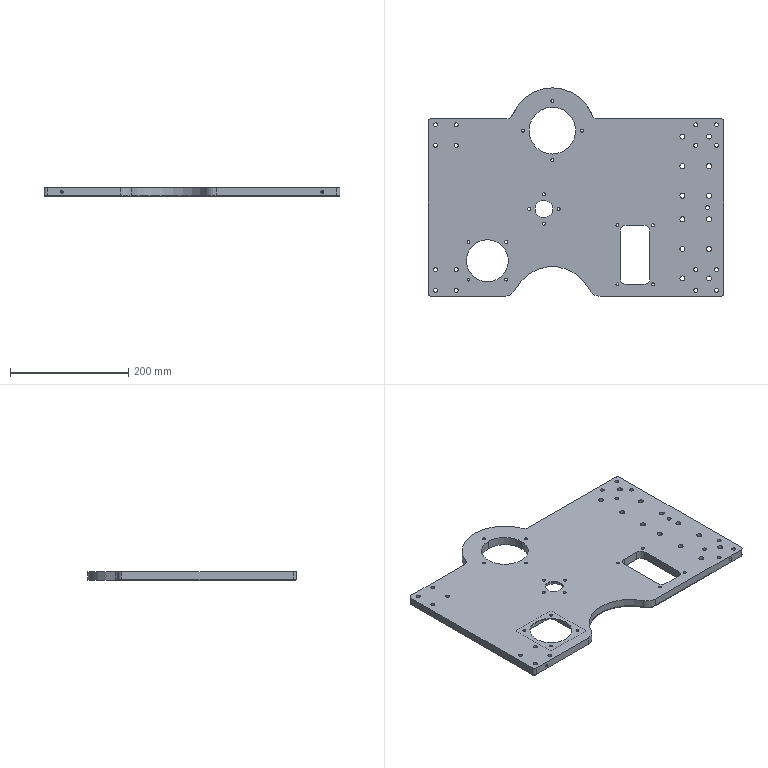NC program | Mastercam | posted with a generic post
Lines 791 to 2246 of 11903:
N7840 T8 M6
N7850 G0 G90 G17 G54 X-172.273 Y94.008 A0. S7000 M3
N7860 G43 H8 Z30. M8
N7870 Z1.3
N7880 G1 Z-.186 F600.
N7890 Y93.977 F4000.
N7900 X-172.242
N7910 G3 X-171.417 Y94.802 I0. J.825
N7920 X-171.575 Y95.287 I-.825 J0.
N7930 G1 X-175.989 Y101.367
N7940 G3 X-176.657 Y101.708 I-.668 J-.484
N7950 X-177.482 Y100.883 I0. J-.825
N7960 G1 Y88.768
N7970 X-165.379
N7980 G0 Z30.
N7990 X-127.758 Y93.977
N8000 Z1.3
N8010 G1 Z-.186 F600.
N8020 X-127.727 F4000.
N8030 Y94.008
N8040 G3 X-128.552 Y94.833 I-.825 J0.
N8050 X-129.038 Y94.675 I0. J-.825
N8060 G1 X-135.106 Y90.26
N8070 G3 X-135.446 Y89.593 I.485 J-.667
N8080 X-134.621 Y88.768 I.825 J0.
N8090 G1 X-122.518
N8100 Y100.883
N8110 Y131.599
N8120 Y143.732
N8130 X-134.654
N8140 X-165.346
N8150 X-177.482
N8160 Y131.599
N8170 G2 X-178.129 Y130.793 I-.825 J0.
N8180 G1 X-182.044 Y129.929
N8190 G3 X-182.691 Y129.124 I.178 J-.805
N8200 G1 Y116.25
N8210 Y83.559
N8220 X-117.309
N8230 Y148.941
N8240 X-182.691
N8250 Y129.124
N8260 G2 X-183.338 Y128.318 I-.825 J0.
N8270 G1 X-187.253 Y127.454
N8280 G3 X-187.9 Y126.649 I.178 J-.805
N8290 G1 Y116.25
N8300 Y78.35
N8310 X-112.1
N8320 Y154.15
N8330 X-187.9
N8340 Y126.649
N8350 G0 Z30.
N8360 X-172.273 Y94.008
N8370 Z.814
N8380 G1 Z-.672 F600.
N8390 Y93.977 F4000.
N8400 X-172.242
N8410 G3 X-171.417 Y94.802 I0. J.825
N8420 X-171.575 Y95.287 I-.825 J0.
N8430 G1 X-175.989 Y101.367
N8440 G3 X-176.657 Y101.708 I-.668 J-.484
N8450 X-177.482 Y100.883 I0. J-.825
N8460 G1 Y88.768
N8470 X-165.379
N8480 G0 Z30.
N8490 X-127.758 Y93.977
N8500 Z.814
N8510 G1 Z-.672 F600.
N8520 X-127.727 F4000.
N8530 Y94.008
N8540 G3 X-128.552 Y94.833 I-.825 J0.
N8550 X-129.038 Y94.675 I0. J-.825
N8560 G1 X-135.106 Y90.26
N8570 G3 X-135.446 Y89.593 I.485 J-.667
N8580 X-134.621 Y88.768 I.825 J0.
N8590 G1 X-122.518
N8600 Y100.883
N8610 Y131.599
N8620 Y143.732
N8630 X-134.654
N8640 X-165.346
N8650 X-177.482
N8660 Y131.599
N8670 G2 X-178.129 Y130.793 I-.825 J0.
N8680 G1 X-182.044 Y129.929
N8690 G3 X-182.691 Y129.124 I.178 J-.805
N8700 G1 Y116.25
N8710 Y83.559
N8720 X-117.309
N8730 Y148.941
N8740 X-182.691
N8750 Y129.124
N8760 G2 X-183.338 Y128.318 I-.825 J0.
N8770 G1 X-187.253 Y127.454
N8780 G3 X-187.9 Y126.649 I.178 J-.805
N8790 G1 Y116.25
N8800 Y78.35
N8810 X-112.1
N8820 Y154.15
N8830 X-187.9
N8840 Y126.649
N8850 G0 Z30.
N8860 X-172.273 Y94.008
N8870 Z.328
N8880 G1 Z-1.159 F600.
N8890 Y93.977 F4000.
N8900 X-172.242
N8910 G3 X-171.417 Y94.802 I0. J.825
N8920 X-171.575 Y95.287 I-.825 J0.
N8930 G1 X-175.989 Y101.367
N8940 G3 X-176.657 Y101.708 I-.668 J-.484
N8950 X-177.482 Y100.883 I0. J-.825
N8960 G1 Y88.768
N8970 X-165.379
N8980 G0 Z30.
N8990 X-127.758 Y93.977
N9000 Z.328
N9010 G1 Z-1.159 F600.
N9020 X-127.727 F4000.
N9030 Y94.008
N9040 G3 X-128.552 Y94.833 I-.825 J0.
N9050 X-129.038 Y94.675 I0. J-.825
N9060 G1 X-135.106 Y90.26
N9070 G3 X-135.446 Y89.593 I.485 J-.667
N9080 X-134.621 Y88.768 I.825 J0.
N9090 G1 X-122.518
N9100 Y100.883
N9110 Y131.599
N9120 Y143.732
N9130 X-134.654
N9140 X-165.346
N9150 X-177.482
N9160 Y131.599
N9170 G2 X-178.129 Y130.793 I-.825 J0.
N9180 G1 X-182.044 Y129.929
N9190 G3 X-182.691 Y129.124 I.178 J-.805
N9200 G1 Y116.25
N9210 Y83.559
N9220 X-117.309
N9230 Y148.941
N9240 X-182.691
N9250 Y129.124
N9260 G2 X-183.338 Y128.318 I-.825 J0.
N9270 G1 X-187.253 Y127.454
N9280 G3 X-187.9 Y126.649 I.178 J-.805
N9290 G1 Y116.25
N9300 Y78.35
N9310 X-112.1
N9320 Y154.15
N9330 X-187.9
N9340 Y126.649
N9350 G0 Z30.
N9360 X-172.273 Y94.008
N9370 Z-.159
N9380 G1 Z-1.645 F600.
N9390 Y93.977 F4000.
N9400 X-172.242
N9410 G3 X-171.417 Y94.802 I0. J.825
N9420 X-171.575 Y95.287 I-.825 J0.
N9430 G1 X-175.989 Y101.367
N9440 G3 X-176.657 Y101.708 I-.668 J-.484
N9450 X-177.482 Y100.883 I0. J-.825
N9460 G1 Y88.768
N9470 X-165.379
N9480 G0 Z30.
N9490 X-127.758 Y93.977
N9500 Z-.159
N9510 G1 Z-1.645 F600.
N9520 X-127.727 F4000.
N9530 Y94.008
N9540 G3 X-128.552 Y94.833 I-.825 J0.
N9550 X-129.038 Y94.675 I0. J-.825
N9560 G1 X-135.106 Y90.26
N9570 G3 X-135.446 Y89.593 I.485 J-.667
N9580 X-134.621 Y88.768 I.825 J0.
N9590 G1 X-122.518
N9600 Y100.883
N9610 Y131.599
N9620 Y143.732
N9630 X-134.654
N9640 X-165.346
N9650 X-177.482
N9660 Y131.599
N9670 G2 X-178.129 Y130.793 I-.825 J0.
N9680 G1 X-182.044 Y129.929
N9690 G3 X-182.691 Y129.124 I.178 J-.805
N9700 G1 Y116.25
N9710 Y83.559
N9720 X-117.309
N9730 Y148.941
N9740 X-182.691
N9750 Y129.124
N9760 G2 X-183.338 Y128.318 I-.825 J0.
N9770 G1 X-187.253 Y127.454
N9780 G3 X-187.9 Y126.649 I.178 J-.805
N9790 G1 Y116.25
N9800 Y78.35
N9810 X-112.1
N9820 Y154.15
N9830 X-187.9
N9840 Y126.649
N9850 G0 Z30.
N9860 X-172.273 Y94.008
N9870 Z-.645
N9880 G1 Z-2.131 F600.
N9890 Y93.977 F4000.
N9900 X-172.242
N9910 G3 X-171.417 Y94.802 I0. J.825
N9920 X-171.575 Y95.287 I-.825 J0.
N9930 G1 X-175.989 Y101.367
N9940 G3 X-176.657 Y101.708 I-.668 J-.484
N9950 X-177.482 Y100.883 I0. J-.825
N9960 G1 Y88.768
N9970 X-165.379
N9980 G0 Z30.
N9990 X-127.758 Y93.977
N100 Z-.645
N110 G1 Z-2.131 F600.
N120 X-127.727 F4000.
N130 Y94.008
N140 G3 X-128.552 Y94.833 I-.825 J0.
N150 X-129.038 Y94.675 I0. J-.825
N160 G1 X-135.106 Y90.26
N170 G3 X-135.446 Y89.593 I.485 J-.667
N180 X-134.621 Y88.768 I.825 J0.
N190 G1 X-122.518
N200 Y100.883
N210 Y131.599
N220 Y143.732
N230 X-134.654
N240 X-165.346
N250 X-177.482
N260 Y131.599
N270 G2 X-178.129 Y130.793 I-.825 J0.
N280 G1 X-182.044 Y129.929
N290 G3 X-182.691 Y129.124 I.178 J-.805
N300 G1 Y116.25
N310 Y83.559
N320 X-117.309
N330 Y148.941
N340 X-182.691
N350 Y129.124
N360 G2 X-183.338 Y128.318 I-.825 J0.
N370 G1 X-187.253 Y127.454
N380 G3 X-187.9 Y126.649 I.178 J-.805
N390 G1 Y116.25
N400 Y78.35
N410 X-112.1
N420 Y154.15
N430 X-187.9
N440 Y126.649
N450 G0 Z30.
N460 X-172.273 Y94.008
N470 Z-1.131
N480 G1 Z-2.617 F600.
N490 Y93.977 F4000.
N500 X-172.242
N510 G3 X-171.417 Y94.802 I0. J.825
N520 X-171.575 Y95.287 I-.825 J0.
N530 G1 X-175.989 Y101.367
N540 G3 X-176.657 Y101.708 I-.668 J-.484
N550 X-177.482 Y100.883 I0. J-.825
N560 G1 Y88.768
N570 X-165.379
N580 G0 Z30.
N590 X-127.758 Y93.977
N600 Z-1.131
N610 G1 Z-2.617 F600.
N620 X-127.727 F4000.
N630 Y94.008
N640 G3 X-128.552 Y94.833 I-.825 J0.
N650 X-129.038 Y94.675 I0. J-.825
N660 G1 X-135.106 Y90.26
N670 G3 X-135.446 Y89.593 I.485 J-.667
N680 X-134.621 Y88.768 I.825 J0.
N690 G1 X-122.518
N700 Y100.883
N710 Y131.599
N720 Y143.732
N730 X-134.654
N740 X-165.346
N750 X-177.482
N760 Y131.599
N770 G2 X-178.129 Y130.793 I-.825 J0.
N780 G1 X-182.044 Y129.929
N790 G3 X-182.691 Y129.124 I.178 J-.805
N800 G1 Y116.25
N810 Y83.559
N820 X-117.309
N830 Y148.941
N840 X-182.691
N850 Y129.124
N860 G2 X-183.338 Y128.318 I-.825 J0.
N870 G1 X-187.253 Y127.454
N880 G3 X-187.9 Y126.649 I.178 J-.805
N890 G1 Y116.25
N900 Y78.35
N910 X-112.1
N920 Y154.15
N930 X-187.9
N940 Y126.649
N950 G0 Z30.
N960 X-172.273 Y94.008
N970 Z-1.617
N980 G1 Z-3.103 F600.
N990 Y93.977 F4000.
N1000 X-172.242
N1010 G3 X-171.417 Y94.802 I0. J.825
N1020 X-171.575 Y95.287 I-.825 J0.
N1030 G1 X-175.989 Y101.367
N1040 G3 X-176.657 Y101.708 I-.668 J-.484
N1050 X-177.482 Y100.883 I0. J-.825
N1060 G1 Y88.768
N1070 X-165.379
N1080 G0 Z30.
N1090 X-127.758 Y93.977
N1100 Z-1.617
N1110 G1 Z-3.103 F600.
N1120 X-127.727 F4000.
N1130 Y94.008
N1140 G3 X-128.552 Y94.833 I-.825 J0.
N1150 X-129.038 Y94.675 I0. J-.825
N1160 G1 X-135.106 Y90.26
N1170 G3 X-135.446 Y89.593 I.485 J-.667
N1180 X-134.621 Y88.768 I.825 J0.
N1190 G1 X-122.518
N1200 Y100.883
N1210 Y131.599
N1220 Y143.732
N1230 X-134.654
N1240 X-165.346
N1250 X-177.482
N1260 Y131.599
N1270 G2 X-178.129 Y130.793 I-.825 J0.
N1280 G1 X-182.044 Y129.929
N1290 G3 X-182.691 Y129.124 I.178 J-.805
N1300 G1 Y116.25
N1310 Y83.559
N1320 X-117.309
N1330 Y148.941
N1340 X-182.691
N1350 Y129.124
N1360 G2 X-183.338 Y128.318 I-.825 J0.
N1370 G1 X-187.253 Y127.454
N1380 G3 X-187.9 Y126.649 I.178 J-.805
N1390 G1 Y116.25
N1400 Y78.35
N1410 X-112.1
N1420 Y154.15
N1430 X-187.9
N1440 Y126.649
N1450 G0 Z30.
N1460 X-172.273 Y94.008
N1470 Z-2.103
N1480 G1 Z-3.59 F600.
N1490 Y93.977 F4000.
N1500 X-172.242
N1510 G3 X-171.417 Y94.802 I0. J.825
N1520 X-171.575 Y95.287 I-.825 J0.
N1530 G1 X-175.989 Y101.367
N1540 G3 X-176.657 Y101.708 I-.668 J-.484
N1550 X-177.482 Y100.883 I0. J-.825
N1560 G1 Y88.768
N1570 X-165.379
N1580 G0 Z30.
N1590 X-127.758 Y93.977
N1600 Z-2.103
N1610 G1 Z-3.59 F600.
N1620 X-127.727 F4000.
N1630 Y94.008
N1640 G3 X-128.552 Y94.833 I-.825 J0.
N1650 X-129.038 Y94.675 I0. J-.825
N1660 G1 X-135.106 Y90.26
N1670 G3 X-135.446 Y89.593 I.485 J-.667
N1680 X-134.621 Y88.768 I.825 J0.
N1690 G1 X-122.518
N1700 Y100.883
N1710 Y131.599
N1720 Y143.732
N1730 X-134.654
N1740 X-165.346
N1750 X-177.482
N1760 Y131.599
N1770 G2 X-178.129 Y130.793 I-.825 J0.
N1780 G1 X-182.044 Y129.929
N1790 G3 X-182.691 Y129.124 I.178 J-.805
N1800 G1 Y116.25
N1810 Y83.559
N1820 X-117.309
N1830 Y148.941
N1840 X-182.691
N1850 Y129.124
N1860 G2 X-183.338 Y128.318 I-.825 J0.
N1870 G1 X-187.253 Y127.454
N1880 G3 X-187.9 Y126.649 I.178 J-.805
N1890 G1 Y116.25
N1900 Y78.35
N1910 X-112.1
N1920 Y154.15
N1930 X-187.9
N1940 Y126.649
N1950 G0 Z30.
N1960 X-172.273 Y94.008
N1970 Z-2.59
N1980 G1 Z-4.076 F600.
N1990 Y93.977 F4000.
N2000 X-172.242
N2010 G3 X-171.417 Y94.802 I0. J.825
N2020 X-171.575 Y95.287 I-.825 J0.
N2030 G1 X-175.989 Y101.367
N2040 G3 X-176.657 Y101.708 I-.668 J-.484
N2050 X-177.482 Y100.883 I0. J-.825
N2060 G1 Y88.768
N2070 X-165.379
N2080 G0 Z30.
N2090 X-127.758 Y93.977
N2100 Z-2.59
N2110 G1 Z-4.076 F600.
N2120 X-127.727 F4000.
N2130 Y94.008
N2140 G3 X-128.552 Y94.833 I-.825 J0.
N2150 X-129.038 Y94.675 I0. J-.825
N2160 G1 X-135.106 Y90.26
N2170 G3 X-135.446 Y89.593 I.485 J-.667
N2180 X-134.621 Y88.768 I.825 J0.
N2190 G1 X-122.518
N2200 Y100.883
N2210 Y131.599
N2220 Y143.732
N2230 X-134.654
N2240 X-165.346
N2250 X-177.482
N2260 Y131.599
N2270 G2 X-178.129 Y130.793 I-.825 J0.
N2280 G1 X-182.044 Y129.929
N2290 G3 X-182.691 Y129.124 I.178 J-.805
N2300 G1 Y116.25
N2310 Y83.559
N2320 X-117.309
N2330 Y148.941
N2340 X-182.691
N2350 Y129.124
N2360 G2 X-183.338 Y128.318 I-.825 J0.
N2370 G1 X-187.253 Y127.454
N2380 G3 X-187.9 Y126.649 I.178 J-.805
N2390 G1 Y116.25
N2400 Y78.35
N2410 X-112.1
N2420 Y154.15
N2430 X-187.9
N2440 Y126.649
N2450 G0 Z30.
N2460 X-172.273 Y94.008
N2470 Z-3.076
N2480 G1 Z-4.562 F600.
N2490 Y93.977 F4000.
N2500 X-172.242
N2510 G3 X-171.417 Y94.802 I0. J.825
N2520 X-171.575 Y95.287 I-.825 J0.
N2530 G1 X-175.989 Y101.367
N2540 G3 X-176.657 Y101.708 I-.668 J-.484
N2550 X-177.482 Y100.883 I0. J-.825
N2560 G1 Y88.768
N2570 X-165.379
N2580 G0 Z30.
N2590 X-127.758 Y93.977
N2600 Z-3.076
N2610 G1 Z-4.562 F600.
N2620 X-127.727 F4000.
N2630 Y94.008
N2640 G3 X-128.552 Y94.833 I-.825 J0.
N2650 X-129.038 Y94.675 I0. J-.825
N2660 G1 X-135.106 Y90.26
N2670 G3 X-135.446 Y89.593 I.485 J-.667
N2680 X-134.621 Y88.768 I.825 J0.
N2690 G1 X-122.518
N2700 Y100.883
N2710 Y131.599
N2720 Y143.732
N2730 X-134.654
N2740 X-165.346
N2750 X-177.482
N2760 Y131.599
N2770 G2 X-178.129 Y130.793 I-.825 J0.
N2780 G1 X-182.044 Y129.929
N2790 G3 X-182.691 Y129.124 I.178 J-.805
N2800 G1 Y116.25
N2810 Y83.559
N2820 X-117.309
N2830 Y148.941
N2840 X-182.691
N2850 Y129.124
N2860 G2 X-183.338 Y128.318 I-.825 J0.
N2870 G1 X-187.253 Y127.454
N2880 G3 X-187.9 Y126.649 I.178 J-.805
N2890 G1 Y116.25
N2900 Y78.35
N2910 X-112.1
N2920 Y154.15
N2930 X-187.9
N2940 Y126.649
N2950 G0 Z30.
N2960 X-172.273 Y94.008
N2970 Z-3.562
N2980 G1 Z-5.048 F600.
N2990 Y93.977 F4000.
N3000 X-172.242
N3010 G3 X-171.417 Y94.802 I0. J.825
N3020 X-171.575 Y95.287 I-.825 J0.
N3030 G1 X-175.989 Y101.367
N3040 G3 X-176.657 Y101.708 I-.668 J-.484
N3050 X-177.482 Y100.883 I0. J-.825
N3060 G1 Y88.768
N3070 X-165.379
N3080 G0 Z30.
N3090 X-127.758 Y93.977
N3100 Z-3.562
N3110 G1 Z-5.048 F600.
N3120 X-127.727 F4000.
N3130 Y94.008
N3140 G3 X-128.552 Y94.833 I-.825 J0.
N3150 X-129.038 Y94.675 I0. J-.825
N3160 G1 X-135.106 Y90.26
N3170 G3 X-135.446 Y89.593 I.485 J-.667
N3180 X-134.621 Y88.768 I.825 J0.
N3190 G1 X-122.518
N3200 Y100.883
N3210 Y131.599
N3220 Y143.732
N3230 X-134.654
N3240 X-165.346
N3250 X-177.482
N3260 Y131.599
N3270 G2 X-178.129 Y130.793 I-.825 J0.
N3280 G1 X-182.044 Y129.929
N3290 G3 X-182.691 Y129.124 I.178 J-.805
N3300 G1 Y116.25
N3310 Y83.559
N3320 X-117.309
N3330 Y148.941
N3340 X-182.691
N3350 Y129.124
N3360 G2 X-183.338 Y128.318 I-.825 J0.
N3370 G1 X-187.253 Y127.454
N3380 G3 X-187.9 Y126.649 I.178 J-.805
N3390 G1 Y116.25
N3400 Y78.35
N3410 X-112.1
N3420 Y154.15
N3430 X-187.9
N3440 Y126.649
N3450 G0 Z30.
N3460 X-172.273 Y94.008
N3470 Z-4.048
N3480 G1 Z-5.534 F600.
N3490 Y93.977 F4000.
N3500 X-172.242
N3510 G3 X-171.417 Y94.802 I0. J.825
N3520 X-171.575 Y95.287 I-.825 J0.
N3530 G1 X-175.989 Y101.367
N3540 G3 X-176.657 Y101.708 I-.668 J-.484
N3550 X-177.482 Y100.883 I0. J-.825
N3560 G1 Y88.768
N3570 X-165.379
N3580 G0 Z30.
N3590 X-127.758 Y93.977
N3600 Z-4.048
N3610 G1 Z-5.534 F600.
N3620 X-127.727 F4000.
N3630 Y94.008
N3640 G3 X-128.552 Y94.833 I-.825 J0.
N3650 X-129.038 Y94.675 I0. J-.825
N3660 G1 X-135.106 Y90.26
N3670 G3 X-135.446 Y89.593 I.485 J-.667
N3680 X-134.621 Y88.768 I.825 J0.
N3690 G1 X-122.518
N3700 Y100.883
N3710 Y131.599
N3720 Y143.732
N3730 X-134.654
N3740 X-165.346
N3750 X-177.482
N3760 Y131.599
N3770 G2 X-178.129 Y130.793 I-.825 J0.
N3780 G1 X-182.044 Y129.929
N3790 G3 X-182.691 Y129.124 I.178 J-.805
N3800 G1 Y116.25
N3810 Y83.559
N3820 X-117.309
N3830 Y148.941
N3840 X-182.691
N3850 Y129.124
N3860 G2 X-183.338 Y128.318 I-.825 J0.
N3870 G1 X-187.253 Y127.454
N3880 G3 X-187.9 Y126.649 I.178 J-.805
N3890 G1 Y116.25
N3900 Y78.35
N3910 X-112.1
N3920 Y154.15
N3930 X-187.9
N3940 Y126.649
N3950 G0 Z30.
N3960 X-172.273 Y94.008
N3970 Z-4.534
N3980 G1 Z-6.021 F600.
N3990 Y93.977 F4000.
N4000 X-172.242
N4010 G3 X-171.417 Y94.802 I0. J.825
N4020 X-171.575 Y95.287 I-.825 J0.
N4030 G1 X-175.989 Y101.367
N4040 G3 X-176.657 Y101.708 I-.668 J-.484
N4050 X-177.482 Y100.883 I0. J-.825
N4060 G1 Y88.768
N4070 X-165.379
N4080 G0 Z30.
N4090 X-127.758 Y93.977
N4100 Z-4.534
N4110 G1 Z-6.021 F600.
N4120 X-127.727 F4000.
N4130 Y94.008
N4140 G3 X-128.552 Y94.833 I-.825 J0.
N4150 X-129.038 Y94.675 I0. J-.825
N4160 G1 X-135.106 Y90.26
N4170 G3 X-135.446 Y89.593 I.485 J-.667
N4180 X-134.621 Y88.768 I.825 J0.
N4190 G1 X-122.518
N4200 Y100.883
N4210 Y131.599
N4220 Y143.732
N4230 X-134.654
N4240 X-165.346
N4250 X-177.482
N4260 Y131.599
N4270 G2 X-178.129 Y130.793 I-.825 J0.
N4280 G1 X-182.044 Y129.929
N4290 G3 X-182.691 Y129.124 I.178 J-.805
N4300 G1 Y116.25
N4310 Y83.559
N4320 X-117.309
N4330 Y148.941
N4340 X-182.691
N4350 Y129.124
N4360 G2 X-183.338 Y128.318 I-.825 J0.
N4370 G1 X-187.253 Y127.454
N4380 G3 X-187.9 Y126.649 I.178 J-.805
N4390 G1 Y116.25
N4400 Y78.35
N4410 X-112.1
N4420 Y154.15
N4430 X-187.9
N4440 Y126.649
N4450 G0 Z30.
N4460 X-172.273 Y94.008
N4470 Z-5.021
N4480 G1 Z-6.507 F600.
N4490 Y93.977 F4000.
N4500 X-172.242
N4510 G3 X-171.417 Y94.802 I0. J.825
N4520 X-171.575 Y95.287 I-.825 J0.
N4530 G1 X-175.989 Y101.367
N4540 G3 X-176.657 Y101.708 I-.668 J-.484
N4550 X-177.482 Y100.883 I0. J-.825
N4560 G1 Y88.768
N4570 X-165.379
N4580 G0 Z30.
N4590 X-127.758 Y93.977
N4600 Z-5.021
N4610 G1 Z-6.507 F600.
N4620 X-127.727 F4000.
N4630 Y94.008
N4640 G3 X-128.552 Y94.833 I-.825 J0.
N4650 X-129.038 Y94.675 I0. J-.825
N4660 G1 X-135.106 Y90.26
N4670 G3 X-135.446 Y89.593 I.485 J-.667
N4680 X-134.621 Y88.768 I.825 J0.
N4690 G1 X-122.518
N4700 Y100.883
N4710 Y131.599
N4720 Y143.732
N4730 X-134.654
N4740 X-165.346
N4750 X-177.482
N4760 Y131.599
N4770 G2 X-178.129 Y130.793 I-.825 J0.
N4780 G1 X-182.044 Y129.929
N4790 G3 X-182.691 Y129.124 I.178 J-.805
N4800 G1 Y116.25
N4810 Y83.559
N4820 X-117.309
N4830 Y148.941
N4840 X-182.691
N4850 Y129.124
N4860 G2 X-183.338 Y128.318 I-.825 J0.
N4870 G1 X-187.253 Y127.454
N4880 G3 X-187.9 Y126.649 I.178 J-.805
N4890 G1 Y116.25
N4900 Y78.35
N4910 X-112.1
N4920 Y154.15
N4930 X-187.9
N4940 Y126.649
N4950 G0 Z30.
N4960 X-172.273 Y94.008
N4970 Z-5.507
N4980 G1 Z-6.993 F600.
N4990 Y93.977 F4000.
N5000 X-172.242
N5010 G3 X-171.417 Y94.802 I0. J.825
N5020 X-171.575 Y95.287 I-.825 J0.
N5030 G1 X-175.989 Y101.367
N5040 G3 X-176.657 Y101.708 I-.668 J-.484
N5050 X-177.482 Y100.883 I0. J-.825
N5060 G1 Y88.768
N5070 X-165.379
N5080 G0 Z30.
N5090 X-127.758 Y93.977
N5100 Z-5.507
N5110 G1 Z-6.993 F600.
N5120 X-127.727 F4000.
N5130 Y94.008
N5140 G3 X-128.552 Y94.833 I-.825 J0.
N5150 X-129.038 Y94.675 I0. J-.825
N5160 G1 X-135.106 Y90.26
N5170 G3 X-135.446 Y89.593 I.485 J-.667
N5180 X-134.621 Y88.768 I.825 J0.
N5190 G1 X-122.518
N5200 Y100.883
N5210 Y131.599
N5220 Y143.732
N5230 X-134.654
N5240 X-165.346
N5250 X-177.482
N5260 Y131.599
N5270 G2 X-178.129 Y130.793 I-.825 J0.
N5280 G1 X-182.044 Y129.929
N5290 G3 X-182.691 Y129.124 I.178 J-.805
N5300 G1 Y116.25
N5310 Y83.559
N5320 X-117.309
N5330 Y148.941
N5340 X-182.691
N5350 Y129.124
N5360 G2 X-183.338 Y128.318 I-.825 J0.
N5370 G1 X-187.253 Y127.454
N5380 G3 X-187.9 Y126.649 I.178 J-.805
N5390 G1 Y116.25
N5400 Y78.35
N5410 X-112.1
N5420 Y154.15
N5430 X-187.9
N5440 Y126.649
N5450 G0 Z30.
N5460 X-172.273 Y94.008
N5470 Z-5.993
N5480 G1 Z-7.479 F600.
N5490 Y93.977 F4000.
N5500 X-172.242
N5510 G3 X-171.417 Y94.802 I0. J.825
N5520 X-171.575 Y95.287 I-.825 J0.
N5530 G1 X-175.989 Y101.367
N5540 G3 X-176.657 Y101.708 I-.668 J-.484
N5550 X-177.482 Y100.883 I0. J-.825
N5560 G1 Y88.768
N5570 X-165.379
N5580 G0 Z30.
N5590 X-127.758 Y93.977
N5600 Z-5.993
N5610 G1 Z-7.479 F600.
N5620 X-127.727 F4000.
N5630 Y94.008
N5640 G3 X-128.552 Y94.833 I-.825 J0.
N5650 X-129.038 Y94.675 I0. J-.825
N5660 G1 X-135.106 Y90.26
N5670 G3 X-135.446 Y89.593 I.485 J-.667
N5680 X-134.621 Y88.768 I.825 J0.
N5690 G1 X-122.518
N5700 Y100.883
N5710 Y131.599
N5720 Y143.732
N5730 X-134.654
N5740 X-165.346
N5750 X-177.482
N5760 Y131.599
N5770 G2 X-178.129 Y130.793 I-.825 J0.
N5780 G1 X-182.044 Y129.929
N5790 G3 X-182.691 Y129.124 I.178 J-.805
N5800 G1 Y116.25
N5810 Y83.559
N5820 X-117.309
N5830 Y148.941
N5840 X-182.691
N5850 Y129.124
N5860 G2 X-183.338 Y128.318 I-.825 J0.
N5870 G1 X-187.253 Y127.454
N5880 G3 X-187.9 Y126.649 I.178 J-.805
N5890 G1 Y116.25
N5900 Y78.35
N5910 X-112.1
N5920 Y154.15
N5930 X-187.9
N5940 Y126.649
N5950 G0 Z30.
N5960 X-172.273 Y94.008
N5970 Z-6.479
N5980 G1 Z-7.966 F600.
N5990 Y93.977 F4000.
N6000 X-172.242
N6010 G3 X-171.417 Y94.802 I0. J.825
N6020 X-171.575 Y95.287 I-.825 J0.
N6030 G1 X-175.989 Y101.367
N6040 G3 X-176.657 Y101.708 I-.668 J-.484
N6050 X-177.482 Y100.883 I0. J-.825
N6060 G1 Y88.768
N6070 X-165.379
N6080 G0 Z30.
N6090 X-127.758 Y93.977
N6100 Z-6.479
N6110 G1 Z-7.966 F600.
N6120 X-127.727 F4000.
N6130 Y94.008
N6140 G3 X-128.552 Y94.833 I-.825 J0.
N6150 X-129.038 Y94.675 I0. J-.825
N6160 G1 X-135.106 Y90.26
N6170 G3 X-135.446 Y89.593 I.485 J-.667
N6180 X-134.621 Y88.768 I.825 J0.
N6190 G1 X-122.518
N6200 Y100.883
N6210 Y131.599
N6220 Y143.732
N6230 X-134.654
N6240 X-165.346
N6250 X-177.482
N6260 Y131.599
N6270 G2 X-178.129 Y130.793 I-.825 J0.
N6280 G1 X-182.044 Y129.929
N6290 G3 X-182.691 Y129.124 I.178 J-.805
N6300 G1 Y116.25
N6310 Y83.559
N6320 X-117.309
N6330 Y148.941
N6340 X-182.691
N6350 Y129.124
N6360 G2 X-183.338 Y128.318 I-.825 J0.
N6370 G1 X-187.253 Y127.454
N6380 G3 X-187.9 Y126.649 I.178 J-.805
N6390 G1 Y116.25
N6400 Y78.35
N6410 X-112.1
N6420 Y154.15
N6430 X-187.9
N6440 Y126.649
N6450 G0 Z30.
N6460 X-172.273 Y94.008
N6470 Z-6.966
N6480 G1 Z-8.452 F600.
N6490 Y93.977 F4000.
N6500 X-172.242
N6510 G3 X-171.417 Y94.802 I0. J.825
N6520 X-171.575 Y95.287 I-.825 J0.
N6530 G1 X-175.989 Y101.367
N6540 G3 X-176.657 Y101.708 I-.668 J-.484
N6550 X-177.482 Y100.883 I0. J-.825
N6560 G1 Y88.768
N6570 X-165.379
N6580 G0 Z30.
N6590 X-127.758 Y93.977
N6600 Z-6.966
N6610 G1 Z-8.452 F600.
N6620 X-127.727 F4000.
N6630 Y94.008
N6640 G3 X-128.552 Y94.833 I-.825 J0.
N6650 X-129.038 Y94.675 I0. J-.825
N6660 G1 X-135.106 Y90.26
N6670 G3 X-135.446 Y89.593 I.485 J-.667
N6680 X-134.621 Y88.768 I.825 J0.
N6690 G1 X-122.518
N6700 Y100.883
N6710 Y131.599
N6720 Y143.732
N6730 X-134.654
N6740 X-165.346
N6750 X-177.482
N6760 Y131.599
N6770 G2 X-178.129 Y130.793 I-.825 J0.
N6780 G1 X-182.044 Y129.929
N6790 G3 X-182.691 Y129.124 I.178 J-.805
N6800 G1 Y116.25
N6810 Y83.559
N6820 X-117.309
N6830 Y148.941
N6840 X-182.691
N6850 Y129.124
N6860 G2 X-183.338 Y128.318 I-.825 J0.
N6870 G1 X-187.253 Y127.454
N6880 G3 X-187.9 Y126.649 I.178 J-.805
N6890 G1 Y116.25
N6900 Y78.35
N6910 X-112.1
N6920 Y154.15
N6930 X-187.9
N6940 Y126.649
N6950 G0 Z30.
N6960 X-172.273 Y94.008
N6970 Z-7.452
N6980 G1 Z-8.938 F600.
N6990 Y93.977 F4000.
N7000 X-172.242
N7010 G3 X-171.417 Y94.802 I0. J.825
N7020 X-171.575 Y95.287 I-.825 J0.
N7030 G1 X-175.989 Y101.367
N7040 G3 X-176.657 Y101.708 I-.668 J-.484
N7050 X-177.482 Y100.883 I0. J-.825
N7060 G1 Y88.768
N7070 X-165.379
N7080 G0 Z30.
N7090 X-127.758 Y93.977
N7100 Z-7.452
N7110 G1 Z-8.938 F600.
N7120 X-127.727 F4000.
N7130 Y94.008
N7140 G3 X-128.552 Y94.833 I-.825 J0.
N7150 X-129.038 Y94.675 I0. J-.825
N7160 G1 X-135.106 Y90.26
N7170 G3 X-135.446 Y89.593 I.485 J-.667
N7180 X-134.621 Y88.768 I.825 J0.
N7190 G1 X-122.518
N7200 Y100.883
N7210 Y131.599
N7220 Y143.732
N7230 X-134.654
N7240 X-165.346
N7250 X-177.482
N7260 Y131.599
N7270 G2 X-178.129 Y130.793 I-.825 J0.
N7280 G1 X-182.044 Y129.929
N7290 G3 X-182.691 Y129.124 I.178 J-.805
N7300 G1 Y116.25
N7310 Y83.559
N7320 X-117.309
N7330 Y148.941
N7340 X-182.691
N7350 Y129.124
N7360 G2 X-183.338 Y128.318 I-.825 J0.
N7370 G1 X-187.253 Y127.454
N7380 G3 X-187.9 Y126.649 I.178 J-.805
N7390 G1 Y116.25
N7400 Y78.35
N7410 X-112.1
N7420 Y154.15
N7430 X-187.9
N7440 Y126.649
N7450 G0 Z30.
N7460 X-172.273 Y94.008
N7470 Z-7.938
N7480 G1 Z-9.424 F600.
N7490 Y93.977 F4000.
N7500 X-172.242
N7510 G3 X-171.417 Y94.802 I0. J.825
N7520 X-171.575 Y95.287 I-.825 J0.
N7530 G1 X-175.989 Y101.367
N7540 G3 X-176.657 Y101.708 I-.668 J-.484
N7550 X-177.482 Y100.883 I0. J-.825
N7560 G1 Y88.768
N7570 X-165.379
N7580 G0 Z30.
N7590 X-127.758 Y93.977
N7600 Z-7.938
N7610 G1 Z-9.424 F600.
N7620 X-127.727 F4000.
N7630 Y94.008
N7640 G3 X-128.552 Y94.833 I-.825 J0.
N7650 X-129.038 Y94.675 I0. J-.825
N7660 G1 X-135.106 Y90.26
N7670 G3 X-135.446 Y89.593 I.485 J-.667
N7680 X-134.621 Y88.768 I.825 J0.
N7690 G1 X-122.518
N7700 Y100.883
N7710 Y131.599
N7720 Y143.732
N7730 X-134.654
N7740 X-165.346
N7750 X-177.482
N7760 Y131.599
N7770 G2 X-178.129 Y130.793 I-.825 J0.
N7780 G1 X-182.044 Y129.929
N7790 G3 X-182.691 Y129.124 I.178 J-.805
N7800 G1 Y116.25
N7810 Y83.559
N7820 X-117.309
N7830 Y148.941
N7840 X-182.691
N7850 Y129.124
N7860 G2 X-183.338 Y128.318 I-.825 J0.
N7870 G1 X-187.253 Y127.454
N7880 G3 X-187.9 Y126.649 I.178 J-.805
N7890 G1 Y116.25
N7900 Y78.35
N7910 X-112.1
N7920 Y154.15
N7930 X-187.9
N7940 Y126.649
N7950 G0 Z30.
N7960 X-172.273 Y94.008
N7970 Z-8.424
N7980 G1 Z-9.91 F600.
N7990 Y93.977 F4000.
N8000 X-172.242
N8010 G3 X-171.417 Y94.802 I0. J.825
N8020 X-171.575 Y95.287 I-.825 J0.
N8030 G1 X-175.989 Y101.367
N8040 G3 X-176.657 Y101.708 I-.668 J-.484
N8050 X-177.482 Y100.883 I0. J-.825
N8060 G1 Y88.768
N8070 X-165.379
N8080 G0 Z30.
N8090 X-127.758 Y93.977
N8100 Z-8.424
N8110 G1 Z-9.91 F600.
N8120 X-127.727 F4000.
N8130 Y94.008
N8140 G3 X-128.552 Y94.833 I-.825 J0.
N8150 X-129.038 Y94.675 I0. J-.825
N8160 G1 X-135.106 Y90.26
N8170 G3 X-135.446 Y89.593 I.485 J-.667
N8180 X-134.621 Y88.768 I.825 J0.
N8190 G1 X-122.518
N8200 Y100.883
N8210 Y131.599
N8220 Y143.732
N8230 X-134.654
N8240 X-165.346
N8250 X-177.482
N8260 Y131.599
N8270 G2 X-178.129 Y130.793 I-.825 J0.
N8280 G1 X-182.044 Y129.929
N8290 G3 X-182.691 Y129.124 I.178 J-.805
N8300 G1 Y116.25
N8310 Y83.559
N8320 X-117.309
N8330 Y148.941
N8340 X-182.691
N8350 Y129.124
N8360 G2 X-183.338 Y128.318 I-.825 J0.
N8370 G1 X-187.253 Y127.454
N8380 G3 X-187.9 Y126.649 I.178 J-.805
N8390 G1 Y116.25
N8400 Y78.35
N8410 X-112.1
N8420 Y154.15
N8430 X-187.9
N8440 Y126.649
N8450 G0 Z30.
N8460 X-172.273 Y94.008
N8470 Z-8.91
N8480 G1 Z-10.397 F600.
N8490 Y93.977 F4000.
N8500 X-172.242
N8510 G3 X-171.417 Y94.802 I0. J.825
N8520 X-171.575 Y95.287 I-.825 J0.
N8530 G1 X-175.989 Y101.367
N8540 G3 X-176.657 Y101.708 I-.668 J-.484
N8550 X-177.482 Y100.883 I0. J-.825
N8560 G1 Y88.768
N8570 X-165.379
N8580 G0 Z30.
N8590 X-127.758 Y93.977
N8600 Z-8.91
N8610 G1 Z-10.397 F600.
N8620 X-127.727 F4000.
N8630 Y94.008
N8640 G3 X-128.552 Y94.833 I-.825 J0.
N8650 X-129.038 Y94.675 I0. J-.825
N8660 G1 X-135.106 Y90.26
N8670 G3 X-135.446 Y89.593 I.485 J-.667
N8680 X-134.621 Y88.768 I.825 J0.
N8690 G1 X-122.518
N8700 Y100.883
N8710 Y131.599
N8720 Y143.732
N8730 X-134.654
N8740 X-165.346
N8750 X-177.482
N8760 Y131.599
N8770 G2 X-178.129 Y130.793 I-.825 J0.
N8780 G1 X-182.044 Y129.929
N8790 G3 X-182.691 Y129.124 I.178 J-.805
N8800 G1 Y116.25
N8810 Y83.559
N8820 X-117.309
N8830 Y148.941
N8840 X-182.691
N8850 Y129.124
N8860 G2 X-183.338 Y128.318 I-.825 J0.
N8870 G1 X-187.253 Y127.454
N8880 G3 X-187.9 Y126.649 I.178 J-.805
N8890 G1 Y116.25
N8900 Y78.35
N8910 X-112.1
N8920 Y154.15
N8930 X-187.9
N8940 Y126.649
N8950 G0 Z30.
N8960 X-172.273 Y94.008
N8970 Z-9.397
N8980 G1 Z-10.883 F600.
N8990 Y93.977 F4000.
N9000 X-172.242
N9010 G3 X-171.417 Y94.802 I0. J.825
N9020 X-171.575 Y95.287 I-.825 J0.
N9030 G1 X-175.989 Y101.367
N9040 G3 X-176.657 Y101.708 I-.668 J-.484
N9050 X-177.482 Y100.883 I0. J-.825
N9060 G1 Y88.768
N9070 X-165.379
N9080 G0 Z30.
N9090 X-127.758 Y93.977
N9100 Z-9.397
N9110 G1 Z-10.883 F600.
N9120 X-127.727 F4000.
N9130 Y94.008
N9140 G3 X-128.552 Y94.833 I-.825 J0.
N9150 X-129.038 Y94.675 I0. J-.825
N9160 G1 X-135.106 Y90.26
N9170 G3 X-135.446 Y89.593 I.485 J-.667
N9180 X-134.621 Y88.768 I.825 J0.
N9190 G1 X-122.518
N9200 Y100.883
N9210 Y131.599
N9220 Y143.732
N9230 X-134.654
N9240 X-165.346
N9250 X-177.482
N9260 Y131.599
N9270 G2 X-178.129 Y130.793 I-.825 J0.
N9280 G1 X-182.044 Y129.929
N9290 G3 X-182.691 Y129.124 I.178 J-.805
N9300 G1 Y116.25
N9310 Y83.559
N9320 X-117.309
N9330 Y148.941
N9340 X-182.691
N9350 Y129.124
N9360 G2 X-183.338 Y128.318 I-.825 J0.
N9370 G1 X-187.253 Y127.454
N9380 G3 X-187.9 Y126.649 I.178 J-.805
N9390 G1 Y116.25
N9400 Y78.35
N9410 X-112.1
N9420 Y154.15
N9430 X-187.9
N9440 Y126.649
N9450 G0 Z30.
N9460 X-172.273 Y94.008
N9470 Z-9.883
N9480 G1 Z-11.369 F600.
N9490 Y93.977 F4000.
N9500 X-172.242
N9510 G3 X-171.417 Y94.802 I0. J.825
N9520 X-171.575 Y95.287 I-.825 J0.
N9530 G1 X-175.989 Y101.367
N9540 G3 X-176.657 Y101.708 I-.668 J-.484
N9550 X-177.482 Y100.883 I0. J-.825
N9560 G1 Y88.768
N9570 X-165.379
N9580 G0 Z30.
N9590 X-127.758 Y93.977
N9600 Z-9.883
N9610 G1 Z-11.369 F600.
N9620 X-127.727 F4000.
N9630 Y94.008
N9640 G3 X-128.552 Y94.833 I-.825 J0.
N9650 X-129.038 Y94.675 I0. J-.825
N9660 G1 X-135.106 Y90.26
N9670 G3 X-135.446 Y89.593 I.485 J-.667
N9680 X-134.621 Y88.768 I.825 J0.
N9690 G1 X-122.518
N9700 Y100.883
N9710 Y131.599
N9720 Y143.732
N9730 X-134.654
N9740 X-165.346
N9750 X-177.482
N9760 Y131.599
N9770 G2 X-178.129 Y130.793 I-.825 J0.
N9780 G1 X-182.044 Y129.929
N9790 G3 X-182.691 Y129.124 I.178 J-.805
N9800 G1 Y116.25
N9810 Y83.559
N9820 X-117.309
N9830 Y148.941
N9840 X-182.691
N9850 Y129.124
N9860 G2 X-183.338 Y128.318 I-.825 J0.
N9870 G1 X-187.253 Y127.454
N9880 G3 X-187.9 Y126.649 I.178 J-.805
N9890 G1 Y116.25
N9900 Y78.35
N9910 X-112.1
N9920 Y154.15
N9930 X-187.9
N9940 Y126.649
N9950 G0 Z30.
N9960 X-172.273 Y94.008
N9970 Z-10.369
N9980 G1 Z-11.855 F600.
N9990 Y93.977 F4000.
N100 X-172.242
N110 G3 X-171.417 Y94.802 I0. J.825
N120 X-171.575 Y95.287 I-.825 J0.
N130 G1 X-175.989 Y101.367
N140 G3 X-176.657 Y101.708 I-.668 J-.484
N150 X-177.482 Y100.883 I0. J-.825
N160 G1 Y88.768
N170 X-165.379
N180 G0 Z30.
N190 X-127.758 Y93.977
N200 Z-10.369
N210 G1 Z-11.855 F600.
N220 X-127.727 F4000.
N230 Y94.008
N240 G3 X-128.552 Y94.833 I-.825 J0.
N250 X-129.038 Y94.675 I0. J-.825
N260 G1 X-135.106 Y90.26
N270 G3 X-135.446 Y89.593 I.485 J-.667
N280 X-134.621 Y88.768 I.825 J0.
N290 G1 X-122.518
N300 Y100.883
N310 Y131.599
N320 Y143.732
N330 X-134.654
N340 X-165.346
N350 X-177.482
N360 Y131.599
N370 G2 X-178.129 Y130.793 I-.825 J0.
N380 G1 X-182.044 Y129.929
N390 G3 X-182.691 Y129.124 I.178 J-.805
N400 G1 Y116.25
N410 Y83.559
N420 X-117.309
N430 Y148.941
N440 X-182.691
N450 Y129.124
N460 G2 X-183.338 Y128.318 I-.825 J0.
N470 G1 X-187.253 Y127.454
N480 G3 X-187.9 Y126.649 I.178 J-.805
N490 G1 Y116.25
N500 Y78.35
N510 X-112.1
N520 Y154.15
N530 X-187.9
N540 Y126.649
N550 G0 Z30.
N560 X-172.273 Y94.008
N570 Z-10.855
N580 G1 Z-12.341 F600.
N590 Y93.977 F4000.
N600 X-172.242
N610 G3 X-171.417 Y94.802 I0. J.825
N620 X-171.575 Y95.287 I-.825 J0.
N630 G1 X-175.989 Y101.367
N640 G3 X-176.657 Y101.708 I-.668 J-.484
N650 X-177.482 Y100.883 I0. J-.825
N660 G1 Y88.768
N670 X-165.379
N680 G0 Z30.
N690 X-127.758 Y93.977
N700 Z-10.855
N710 G1 Z-12.341 F600.
N720 X-127.727 F4000.
N730 Y94.008
N740 G3 X-128.552 Y94.833 I-.825 J0.
N750 X-129.038 Y94.675 I0. J-.825
N760 G1 X-135.106 Y90.26
N770 G3 X-135.446 Y89.593 I.485 J-.667
N780 X-134.621 Y88.768 I.825 J0.
N790 G1 X-122.518
N800 Y100.883
N810 Y131.599
N820 Y143.732
N830 X-134.654
N840 X-165.346
N850 X-177.482
N860 Y131.599
N870 G2 X-178.129 Y130.793 I-.825 J0.
N880 G1 X-182.044 Y129.929
N890 G3 X-182.691 Y129.124 I.178 J-.805
N900 G1 Y116.25
N910 Y83.559
N920 X-117.309
N930 Y148.941
N940 X-182.691
N950 Y129.124
N960 G2 X-183.338 Y128.318 I-.825 J0.
N970 G1 X-187.253 Y127.454
N980 G3 X-187.9 Y126.649 I.178 J-.805
N990 G1 Y116.25
N1000 Y78.35
N1010 X-112.1
N1020 Y154.15
N1030 X-187.9
N1040 Y126.649
N1050 G0 Z30.
N1060 X-172.273 Y94.008
N1070 Z-11.341
N1080 G1 Z-12.828 F600.
N1090 Y93.977 F4000.
N1100 X-172.242
N1110 G3 X-171.417 Y94.802 I0. J.825
N1120 X-171.575 Y95.287 I-.825 J0.
N1130 G1 X-175.989 Y101.367
N1140 G3 X-176.657 Y101.708 I-.668 J-.484
N1150 X-177.482 Y100.883 I0. J-.825
N1160 G1 Y88.768
N1170 X-165.379
N1180 G0 Z30.
N1190 X-127.758 Y93.977
N1200 Z-11.341
N1210 G1 Z-12.828 F600.
N1220 X-127.727 F4000.
N1230 Y94.008
N1240 G3 X-128.552 Y94.833 I-.825 J0.
N1250 X-129.038 Y94.675 I0. J-.825
N1260 G1 X-135.106 Y90.26
N1270 G3 X-135.446 Y89.593 I.485 J-.667
N1280 X-134.621 Y88.768 I.825 J0.
N1290 G1 X-122.518
N1300 Y100.883
N1310 Y131.599
N1320 Y143.732
N1330 X-134.654
N1340 X-165.346
N1350 X-177.482
N1360 Y131.599
N1370 G2 X-178.129 Y130.793 I-.825 J0.
N1380 G1 X-182.044 Y129.929
N1390 G3 X-182.691 Y129.124 I.178 J-.805
N1400 G1 Y116.25
N1410 Y83.559
N1420 X-117.309
N1430 Y148.941
N1440 X-182.691
N1450 Y129.124
N1460 G2 X-183.338 Y128.318 I-.825 J0.
N1470 G1 X-187.253 Y127.454
N1480 G3 X-187.9 Y126.649 I.178 J-.805
N1490 G1 Y116.25
N1500 Y78.35
N1510 X-112.1
N1520 Y154.15
N1530 X-187.9
N1540 Y126.649
N1550 G0 Z30.
N1560 X-172.273 Y94.008
N1570 Z-11.828
N1580 G1 Z-13.314 F600.
N1590 Y93.977 F4000.
N1600 X-172.242
N1610 G3 X-171.417 Y94.802 I0. J.825
N1620 X-171.575 Y95.287 I-.825 J0.
N1630 G1 X-175.989 Y101.367
N1640 G3 X-176.657 Y101.708 I-.668 J-.484
N1650 X-177.482 Y100.883 I0. J-.825
N1660 G1 Y88.768
N1670 X-165.379
N1680 G0 Z30.
N1690 X-127.758 Y93.977
N1700 Z-11.828
N1710 G1 Z-13.314 F600.
N1720 X-127.727 F4000.
N1730 Y94.008
N1740 G3 X-128.552 Y94.833 I-.825 J0.
N1750 X-129.038 Y94.675 I0. J-.825
N1760 G1 X-135.106 Y90.26
N1770 G3 X-135.446 Y89.593 I.485 J-.667
N1780 X-134.621 Y88.768 I.825 J0.
N1790 G1 X-122.518
N1800 Y100.883
N1810 Y131.599
N1820 Y143.732
N1830 X-134.654
N1840 X-165.346
N1850 X-177.482
N1860 Y131.599
N1870 G2 X-178.129 Y130.793 I-.825 J0.
N1880 G1 X-182.044 Y129.929
N1890 G3 X-182.691 Y129.124 I.178 J-.805
N1900 G1 Y116.25
N1910 Y83.559
N1920 X-117.309
N1930 Y148.941
N1940 X-182.691
N1950 Y129.124
N1960 G2 X-183.338 Y128.318 I-.825 J0.
N1970 G1 X-187.253 Y127.454
N1980 G3 X-187.9 Y126.649 I.178 J-.805
N1990 G1 Y116.25
N2000 Y78.35
N2010 X-112.1
N2020 Y154.15
N2030 X-187.9
N2040 Y126.649
N2050 G0 Z30.
N2060 X-172.273 Y94.008
N2070 Z-12.314
N2080 G1 Z-13.8 F600.
N2090 Y93.977 F4000.
N2100 X-172.242
N2110 G3 X-171.417 Y94.802 I0. J.825
N2120 X-171.575 Y95.287 I-.825 J0.
N2130 G1 X-175.989 Y101.367
N2140 G3 X-176.657 Y101.708 I-.668 J-.484
N2150 X-177.482 Y100.883 I0. J-.825
N2160 G1 Y88.768
N2170 X-165.379
N2180 G0 Z30.
N2190 X-127.758 Y93.977
N2200 Z-12.314
N2210 G1 Z-13.8 F600.
N2220 X-127.727 F4000.
N2230 Y94.008
N2240 G3 X-128.552 Y94.833 I-.825 J0.
N2250 X-129.038 Y94.675 I0. J-.825
N2260 G1 X-135.106 Y90.26
N2270 G3 X-135.446 Y89.593 I.485 J-.667
N2280 X-134.621 Y88.768 I.825 J0.
N2290 G1 X-122.518
N2300 Y100.883
N2310 Y131.599
N2320 Y143.732
N2330 X-134.654
N2340 X-165.346
N2350 X-177.482
N2360 Y131.599
N2370 G2 X-178.129 Y130.793 I-.825 J0.
N2380 G1 X-182.044 Y129.929
N2390 G3 X-182.691 Y129.124 I.178 J-.805
N2400 G1 Y116.25
N2410 Y83.559
N2420 X-117.309
N2430 Y148.941
N2440 X-182.691
N2450 Y129.124
N2460 G2 X-183.338 Y128.318 I-.825 J0.
N2470 G1 X-187.253 Y127.454
N2480 G3 X-187.9 Y126.649 I.178 J-.805
N2490 G1 Y116.25
N2500 Y78.35
N2510 X-112.1
N2520 Y154.15
N2530 X-187.9
N2540 Y126.649
N2550 G0 Z30.
N2560 M5
N2570 G91 G28 Z0. M9
N2580 A0.
N2590 M01